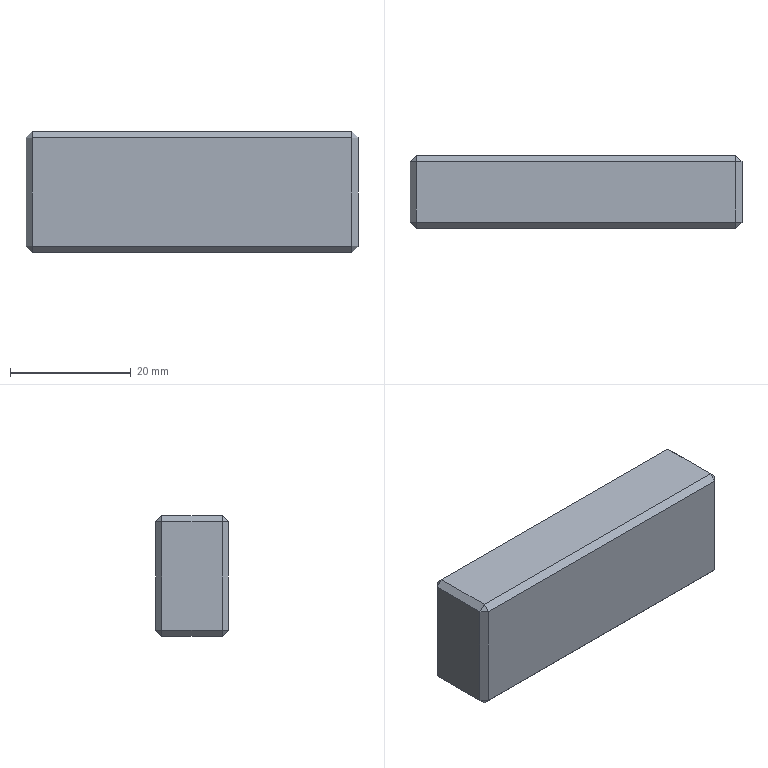Part | STEP file | Cam top plate | 1 solid | 38 faces | box 55 x 12 x 20 mm | volume 12439 mm3 | plane 26 | cone 8 | cylinder 4 | commonest cylinder face diameters 4.917 x4